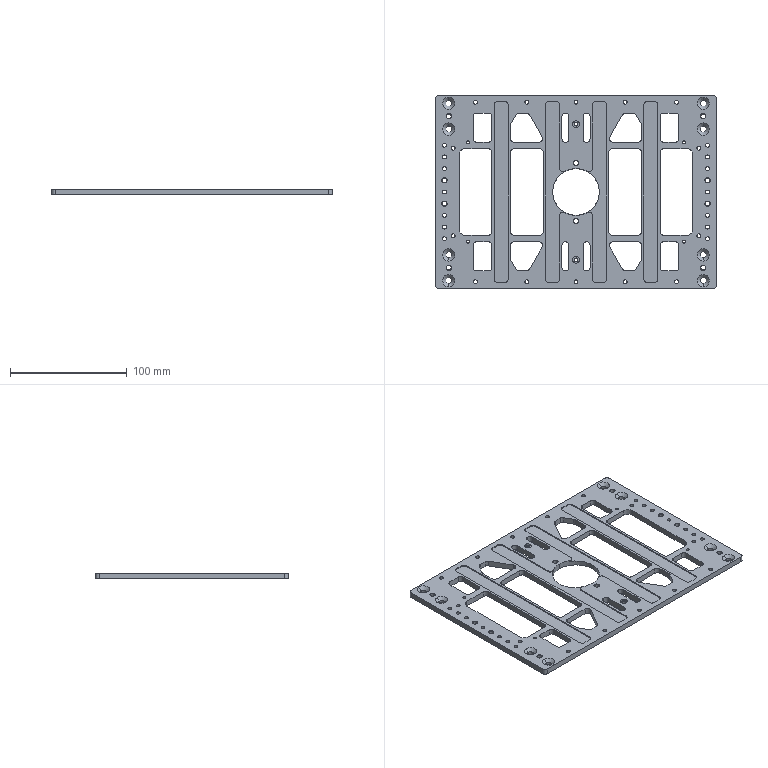CAM job | NX | 3-axis milling, drilling | part box 240 x 165 x 5 mm | stock box 244 x 169 x 5 mm
Tools:
number,name,description,diameter,corner_radius,flute_length,length,flutes
1,D6A45,Milling Tool-5 Parameters,6.0,0.0,50.0,75.0,2
3,3.3ZT,Drilling Tool,3.3,0.0,35.0,50.0,2
2,2.5ZT,Drilling Tool,2.5,0.0,35.0,50.0,2
16,3.2ZT,Drilling Tool,3.2,0.0,35.0,50.0,2
18,3.8ZT,Drilling Tool,3.8,0.0,35.0,50.0,2
9,5.3ZT,Drilling Tool,5.3,0.0,35.0,50.0,2
15,D10,Milling Tool-5 Parameters,10.0,0.0,50.0,75.0,2
14,D10JING,Milling Tool-5 Parameters,10.0,0.0,50.0,75.0,2
11,D4,Milling Tool-5 Parameters,4.0,0.0,50.0,75.0,2
17,D3,Milling Tool-5 Parameters,3.0,0.0,50.0,75.0,2
Operations:
program,operation,operation_type,tool,method,geometry_group,spindle_rpm,surface_speed,feed_per_tooth,feed_cut,feed_plunge,cut_length_mm,path_length_mm,cut_time_min,machine_time_min
1,DRILLING,Operation,D6A45,METHOD,A,5000.0,94.0,0.035,350.0,0.0,212.0,1574.424,0.6057,0.742
1,DRILLING_COPY,Operation,3.3ZT,METHOD,A,2000.0,20.0,0.05,200.0,0.0,293.76,1402.514,1.469,1.58
1,DRILLING_COPY_COPY_1,Operation,3.2ZT,METHOD,A,2000.0,20.0,0.05,200.0,0.0,19.923,218.884,0.0996,0.1195
1,DRILLING_COPY_COPY,Operation,2.5ZT,METHOD,A,2000.0,15.0,0.0375,150.0,0.0,41.004,506.144,0.2734,0.3199
1,DRILLING_COPY_COPY_1_COPY,Operation,3.8ZT,METHOD,A,2000.0,20.0,0.05,200.0,0.0,101.416,831.863,0.5071,0.5801
1,DRILLING_COPY_COPY_1_COPY_COPY,Operation,5.3ZT,METHOD,A,2000.0,20.0,0.05,200.0,0.0,84.738,771.895,0.4237,0.4924
1,ZLEVEL_PROFILE,ZLevelMilling,D10,METHOD,A,9500.0,298.0,0.1579,3000.0,1000.0,5068.288,5129.688,1.72,1.726
1,ZLEVEL_PROFILE_COPY,ZLevelMilling,D10,METHOD,A,9500.0,298.0,0.1579,3000.0,1000.0,2635.884,4242.436,1.133,1.294
1,PLANAR_MILL,PlanarMilling,D10,METHOD,A,9500.0,298.0,0.1579,3000.0,100.0,7629.265,8374.757,2.543,2.618
1,PLANAR_MILL_COPY,PlanarMilling,D10,METHOD,A,9500.0,298.0,0.1579,3000.0,100.0,1457.317,1761.132,0.4858,0.5162
1,PLANAR_MILL_COPY_COPY,PlanarMilling,D10JING,METHOD,A,9500.0,298.0,0.0789,1500.0,100.0,2548.747,2849.278,1.699,1.729
1,ZLEVEL_PROFILE_COPY_COPY,ZLevelMilling,D10JING,METHOD,A,9500.0,298.0,0.0789,1500.0,1000.0,1167.951,4017.067,0.7849,1.07
1,ZLEVEL_PROFILE_COPY_COPY_1,ZLevelMilling,D4,METHOD,A,9500.0,119.0,0.0947,1800.0,1000.0,2623.874,3029.344,1.522,1.562
1,ZLEVEL_PROFILE_COPY_COPY_1_COPY,ZLevelMilling,D4,METHOD,A,9500.0,119.0,0.0947,1800.0,1000.0,5184.29,14209.008,3.236,4.138
1,HOLE_MILLING,CylinderMilling,D4,METHOD,A,9500.0,119.0,0.0789,1500.0,100.0,72.365,309.765,0.0482,0.072
1,PLANAR_MILL_COPY_COPY_COPY,PlanarMilling,D6A45,METHOD,A,9500.0,179.0,0.0658,1250.0,100.0,4567.855,10244.687,3.654,4.222
1,ZLEVEL_PROFILE_COPY_COPY_1_COPY_1,ZLevelMilling,D6A45,METHOD,A,9500.0,179.0,0.0632,1200.0,1000.0,1020.33,2089.948,0.914,1.021
1,ZLEVEL_PROFILE_COPY_COPY_1_COPY_1_COPY,ZLevelMilling,D6A45,METHOD,A,9500.0,179.0,0.0632,1200.0,1000.0,102.132,1229.184,0.0898,0.2025
1,刀补14,PlanarMilling,D10JING,METHOD,A,9500.0,298.0,0.0789,1500.0,100.0,1218.282,1525.524,0.8122,0.8429
1,刀补,CylinderMilling,D3,METHOD,A,9500.0,89.0,0.0658,1250.0,100.0,186.489,1250.906,0.1492,0.2556
1,ZLEVEL_PROFILE_COPY_1,ZLevelMilling,D10JING,METHOD,A,9500.0,298.0,0.0632,1200.0,1000.0,4213.838,4280.138,3.517,3.523